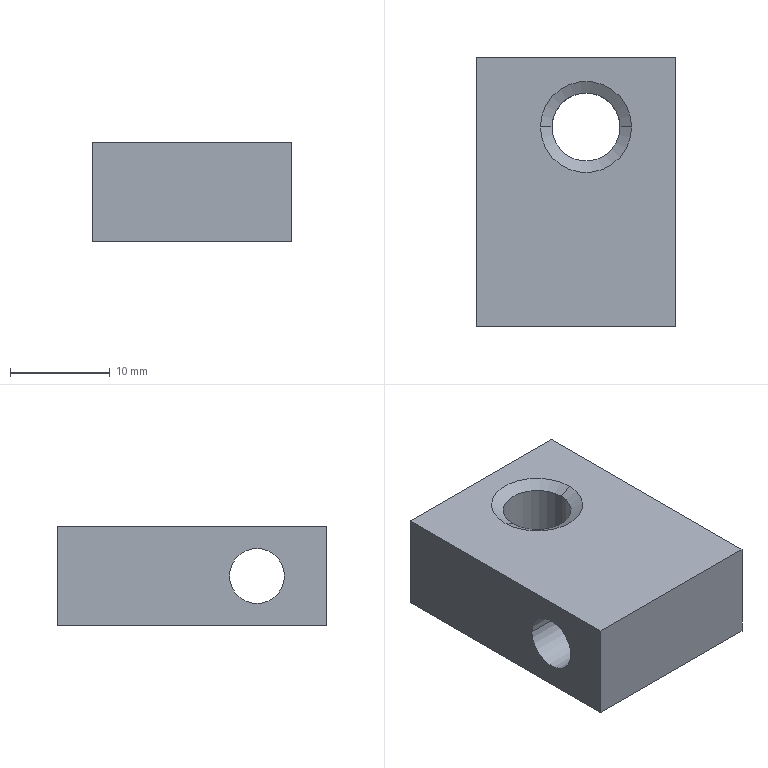Part | NX | 1 solid | 12 faces | box 20 x 27 x 10 mm | volume 4552 mm3 | plane 6 | cylinder 4 | cone 2 | commonest cylinder face diameters 5.5 x2 6.8 x2
STEP:
#1=CARTESIAN_POINT('',(508.,48.4,-222.82));
#2=VERTEX_POINT('',#1);
#3=CARTESIAN_POINT('',(508.,75.4,-222.82));
#4=VERTEX_POINT('',#3);
#5=CARTESIAN_POINT('',(508.,0.,-222.82));
#6=DIRECTION('',(0.,1.,0.));
#7=VECTOR('',#6,1000.);
#8=LINE('',#5,#7);
#9=EDGE_CURVE('',#2,#4,#8,.T.);
#10=ORIENTED_EDGE('',*,*,#9,.F.);
#11=CARTESIAN_POINT('',(528.,48.4,-222.82));
#12=VERTEX_POINT('',#11);
#13=CARTESIAN_POINT('',(0.,48.4,-222.82));
#14=DIRECTION('',(-1.,0.,0.));
#15=VECTOR('',#14,1000.);
#16=LINE('',#13,#15);
#17=EDGE_CURVE('',#12,#2,#16,.T.);
#18=ORIENTED_EDGE('',*,*,#17,.F.);
#19=CARTESIAN_POINT('',(528.,75.4,-222.82));
#20=VERTEX_POINT('',#19);
#21=CARTESIAN_POINT('',(528.,0.,-222.82));
#22=DIRECTION('',(0.,1.,0.));
#23=VECTOR('',#22,1000.);
#24=LINE('',#21,#23);
#25=EDGE_CURVE('',#12,#20,#24,.T.);
#26=ORIENTED_EDGE('',*,*,#25,.T.);
#27=CARTESIAN_POINT('',(0.,75.4,-222.82));
#28=DIRECTION('',(1.,0.,0.));
#29=VECTOR('',#28,1000.);
#30=LINE('',#27,#29);
#31=EDGE_CURVE('',#4,#20,#30,.T.);
#32=ORIENTED_EDGE('',*,*,#31,.F.);
#33=EDGE_LOOP('',(#10,#18,#26,#32));
#34=FACE_BOUND('',#33,.T.);
#35=CARTESIAN_POINT('',(523.562,68.4,-222.82));
#36=VERTEX_POINT('',#35);
#37=CARTESIAN_POINT('',(514.437,68.4,-222.82));
#38=VERTEX_POINT('',#37);
#39=CARTESIAN_POINT('',(519.,68.4,-222.82));
#40=DIRECTION('',(0.,0.,1.));
#41=DIRECTION('',(1.,0.,0.));
#42=AXIS2_PLACEMENT_3D('',#39,#40,#41);
#43=CIRCLE('',#42,4.563);
#44=EDGE_CURVE('',#36,#38,#43,.T.);
#45=ORIENTED_EDGE('',*,*,#44,.F.);
#46=CARTESIAN_POINT('',(519.,68.4,-222.82));
#47=DIRECTION('',(0.,0.,1.));
#48=DIRECTION('',(1.,0.,0.));
#49=AXIS2_PLACEMENT_3D('',#46,#47,#48);
#50=CIRCLE('',#49,4.563);
#51=EDGE_CURVE('',#38,#36,#50,.T.);
#52=ORIENTED_EDGE('',*,*,#51,.F.);
#53=EDGE_LOOP('',(#45,#52));
#54=FACE_BOUND('',#53,.T.);
#55=CARTESIAN_POINT('',(518.,48.4,-222.82));
#56=DIRECTION('',(0.,0.,1.));
#57=DIRECTION('',(1.,0.,0.));
#58=AXIS2_PLACEMENT_3D('',#55,#56,#57);
#59=PLANE('',#58);
#60=ADVANCED_FACE('',(#34,#54),#59,.T.);
#61=CARTESIAN_POINT('',(508.,48.4,-232.82));
#62=VERTEX_POINT('',#61);
#63=CARTESIAN_POINT('',(508.,48.4,-235.336));
#64=DIRECTION('',(0.,0.,1.));
#65=VECTOR('',#64,1000.);
#66=LINE('',#63,#65);
#67=EDGE_CURVE('',#62,#2,#66,.T.);
#68=ORIENTED_EDGE('',*,*,#67,.F.);
#69=CARTESIAN_POINT('',(528.,48.4,-232.82));
#70=VERTEX_POINT('',#69);
#71=CARTESIAN_POINT('',(0.,48.4,-232.82));
#72=DIRECTION('',(1.,0.,0.));
#73=VECTOR('',#72,1000.);
#74=LINE('',#71,#73);
#75=EDGE_CURVE('',#62,#70,#74,.T.);
#76=ORIENTED_EDGE('',*,*,#75,.T.);
#77=CARTESIAN_POINT('',(528.,48.4,-235.336));
#78=DIRECTION('',(0.,0.,1.));
#79=VECTOR('',#78,1000.);
#80=LINE('',#77,#79);
#81=EDGE_CURVE('',#70,#12,#80,.T.);
#82=ORIENTED_EDGE('',*,*,#81,.T.);
#83=ORIENTED_EDGE('',*,*,#17,.T.);
#84=EDGE_LOOP('',(#68,#76,#82,#83));
#85=FACE_BOUND('',#84,.T.);
#86=CARTESIAN_POINT('',(518.,48.4,-232.82));
#87=DIRECTION('',(0.,-1.,0.));
#88=DIRECTION('',(0.,0.,-1.));
#89=AXIS2_PLACEMENT_3D('',#86,#87,#88);
#90=PLANE('',#89);
#91=ADVANCED_FACE('',(#85),#90,.T.);
#92=CARTESIAN_POINT('',(508.,75.4,-232.82));
#93=VERTEX_POINT('',#92);
#94=CARTESIAN_POINT('',(508.,0.,-232.82));
#95=DIRECTION('',(0.,-1.,0.));
#96=VECTOR('',#95,1000.);
#97=LINE('',#94,#96);
#98=EDGE_CURVE('',#93,#62,#97,.T.);
#99=ORIENTED_EDGE('',*,*,#98,.F.);
#100=CARTESIAN_POINT('',(528.,75.4,-232.82));
#101=VERTEX_POINT('',#100);
#102=CARTESIAN_POINT('',(0.,75.4,-232.82));
#103=DIRECTION('',(-1.,0.,0.));
#104=VECTOR('',#103,1000.);
#105=LINE('',#102,#104);
#106=EDGE_CURVE('',#101,#93,#105,.T.);
#107=ORIENTED_EDGE('',*,*,#106,.F.);
#108=CARTESIAN_POINT('',(528.,0.,-232.82));
#109=DIRECTION('',(0.,-1.,0.));
#110=VECTOR('',#109,1000.);
#111=LINE('',#108,#110);
#112=EDGE_CURVE('',#101,#70,#111,.T.);
#113=ORIENTED_EDGE('',*,*,#112,.T.);
#114=ORIENTED_EDGE('',*,*,#75,.F.);
#115=EDGE_LOOP('',(#99,#107,#113,#114));
#116=FACE_BOUND('',#115,.T.);
#117=CARTESIAN_POINT('',(515.6,68.4,-232.82));
#118=VERTEX_POINT('',#117);
#119=CARTESIAN_POINT('',(522.4,68.4,-232.82));
#120=VERTEX_POINT('',#119);
#121=CARTESIAN_POINT('',(519.,68.4,-232.82));
#122=DIRECTION('',(0.,0.,1.));
#123=DIRECTION('',(1.,0.,0.));
#124=AXIS2_PLACEMENT_3D('',#121,#122,#123);
#125=CIRCLE('',#124,3.4);
#126=EDGE_CURVE('',#118,#120,#125,.T.);
#127=ORIENTED_EDGE('',*,*,#126,.T.);
#128=CARTESIAN_POINT('',(519.,68.4,-232.82));
#129=DIRECTION('',(0.,0.,1.));
#130=DIRECTION('',(1.,0.,0.));
#131=AXIS2_PLACEMENT_3D('',#128,#129,#130);
#132=CIRCLE('',#131,3.4);
#133=EDGE_CURVE('',#120,#118,#132,.T.);
#134=ORIENTED_EDGE('',*,*,#133,.T.);
#135=EDGE_LOOP('',(#127,#134));
#136=FACE_BOUND('',#135,.T.);
#137=CARTESIAN_POINT('',(518.,62.4,-232.82));
#138=DIRECTION('',(0.,0.,-1.));
#139=DIRECTION('',(0.,-1.,0.));
#140=AXIS2_PLACEMENT_3D('',#137,#138,#139);
#141=PLANE('',#140);
#142=ADVANCED_FACE('',(#116,#136),#141,.T.);
#143=CARTESIAN_POINT('',(508.,75.4,-235.336));
#144=DIRECTION('',(0.,0.,-1.));
#145=VECTOR('',#144,1000.);
#146=LINE('',#143,#145);
#147=EDGE_CURVE('',#4,#93,#146,.T.);
#148=ORIENTED_EDGE('',*,*,#147,.F.);
#149=ORIENTED_EDGE('',*,*,#31,.T.);
#150=CARTESIAN_POINT('',(528.,75.4,-235.336));
#151=DIRECTION('',(0.,0.,1.));
#152=VECTOR('',#151,1000.);
#153=LINE('',#150,#152);
#154=EDGE_CURVE('',#101,#20,#153,.T.);
#155=ORIENTED_EDGE('',*,*,#154,.F.);
#156=ORIENTED_EDGE('',*,*,#106,.T.);
#157=EDGE_LOOP('',(#148,#149,#155,#156));
#158=FACE_BOUND('',#157,.T.);
#159=CARTESIAN_POINT('',(518.,75.4,-222.82));
#160=DIRECTION('',(0.,1.,0.));
#161=DIRECTION('',(1.,0.,0.));
#162=AXIS2_PLACEMENT_3D('',#159,#160,#161);
#163=PLANE('',#162);
#164=ADVANCED_FACE('',(#158),#163,.T.);
#165=ORIENTED_EDGE('',*,*,#98,.T.);
#166=ORIENTED_EDGE('',*,*,#67,.T.);
#167=ORIENTED_EDGE('',*,*,#9,.T.);
#168=ORIENTED_EDGE('',*,*,#147,.T.);
#169=EDGE_LOOP('',(#165,#166,#167,#168));
#170=FACE_BOUND('',#169,.T.);
#171=CARTESIAN_POINT('',(508.,52.65,-227.82));
#172=VERTEX_POINT('',#171);
#173=CARTESIAN_POINT('',(508.,58.15,-227.82));
#174=VERTEX_POINT('',#173);
#175=CARTESIAN_POINT('',(508.,55.4,-227.82));
#176=DIRECTION('',(-1.,0.,0.));
#177=DIRECTION('',(0.,-1.,0.));
#178=AXIS2_PLACEMENT_3D('',#175,#176,#177);
#179=CIRCLE('',#178,2.75);
#180=EDGE_CURVE('',#172,#174,#179,.T.);
#181=ORIENTED_EDGE('',*,*,#180,.F.);
#182=CARTESIAN_POINT('',(508.,55.4,-227.82));
#183=DIRECTION('',(-1.,0.,0.));
#184=DIRECTION('',(0.,-1.,0.));
#185=AXIS2_PLACEMENT_3D('',#182,#183,#184);
#186=CIRCLE('',#185,2.75);
#187=EDGE_CURVE('',#174,#172,#186,.T.);
#188=ORIENTED_EDGE('',*,*,#187,.F.);
#189=EDGE_LOOP('',(#181,#188));
#190=FACE_BOUND('',#189,.T.);
#191=CARTESIAN_POINT('',(508.,57.102,-235.336));
#192=DIRECTION('',(-1.,0.,0.));
#193=DIRECTION('',(0.,1.,0.));
#194=AXIS2_PLACEMENT_3D('',#191,#192,#193);
#195=PLANE('',#194);
#196=ADVANCED_FACE('',(#170,#190),#195,.T.);
#197=ORIENTED_EDGE('',*,*,#154,.T.);
#198=ORIENTED_EDGE('',*,*,#25,.F.);
#199=ORIENTED_EDGE('',*,*,#81,.F.);
#200=ORIENTED_EDGE('',*,*,#112,.F.);
#201=EDGE_LOOP('',(#197,#198,#199,#200));
#202=FACE_BOUND('',#201,.T.);
#203=CARTESIAN_POINT('',(528.,52.65,-227.82));
#204=VERTEX_POINT('',#203);
#205=CARTESIAN_POINT('',(528.,58.15,-227.82));
#206=VERTEX_POINT('',#205);
#207=CARTESIAN_POINT('',(528.,55.4,-227.82));
#208=DIRECTION('',(-1.,0.,0.));
#209=DIRECTION('',(0.,-1.,0.));
#210=AXIS2_PLACEMENT_3D('',#207,#208,#209);
#211=CIRCLE('',#210,2.75);
#212=EDGE_CURVE('',#204,#206,#211,.T.);
#213=ORIENTED_EDGE('',*,*,#212,.T.);
#214=CARTESIAN_POINT('',(528.,55.4,-227.82));
#215=DIRECTION('',(-1.,0.,0.));
#216=DIRECTION('',(0.,-1.,0.));
#217=AXIS2_PLACEMENT_3D('',#214,#215,#216);
#218=CIRCLE('',#217,2.75);
#219=EDGE_CURVE('',#206,#204,#218,.T.);
#220=ORIENTED_EDGE('',*,*,#219,.T.);
#221=EDGE_LOOP('',(#213,#220));
#222=FACE_BOUND('',#221,.T.);
#223=CARTESIAN_POINT('',(528.,57.102,-235.336));
#224=DIRECTION('',(-1.,0.,0.));
#225=DIRECTION('',(0.,1.,0.));
#226=AXIS2_PLACEMENT_3D('',#223,#224,#225);
#227=PLANE('',#226);
#228=ADVANCED_FACE('',(#202,#222),#227,.F.);
#229=ORIENTED_EDGE('',*,*,#212,.F.);
#230=CARTESIAN_POINT('',(521.2,52.65,-227.82));
#231=DIRECTION('',(-1.,0.,0.));
#232=VECTOR('',#231,1000.);
#233=LINE('',#230,#232);
#234=EDGE_CURVE('',#172,#204,#233,.F.);
#235=ORIENTED_EDGE('',*,*,#234,.F.);
#236=ORIENTED_EDGE('',*,*,#180,.T.);
#237=CARTESIAN_POINT('',(521.2,58.15,-227.82));
#238=DIRECTION('',(-1.,0.,0.));
#239=VECTOR('',#238,1000.);
#240=LINE('',#237,#239);
#241=EDGE_CURVE('',#174,#206,#240,.F.);
#242=ORIENTED_EDGE('',*,*,#241,.T.);
#243=EDGE_LOOP('',(#229,#235,#236,#242));
#244=FACE_BOUND('',#243,.T.);
#245=CARTESIAN_POINT('',(521.2,55.4,-227.82));
#246=DIRECTION('',(-1.,0.,0.));
#247=DIRECTION('',(0.,-1.,0.));
#248=AXIS2_PLACEMENT_3D('',#245,#246,#247);
#249=CYLINDRICAL_SURFACE('',#248,2.75);
#250=ADVANCED_FACE('',(#244),#249,.F.);
#251=ORIENTED_EDGE('',*,*,#126,.F.);
#252=CARTESIAN_POINT('',(515.6,68.4,-223.491));
#253=VERTEX_POINT('',#252);
#254=CARTESIAN_POINT('',(515.6,68.4,-222.82));
#255=DIRECTION('',(0.,0.,1.));
#256=VECTOR('',#255,1000.);
#257=LINE('',#254,#256);
#258=EDGE_CURVE('',#118,#253,#257,.T.);
#259=ORIENTED_EDGE('',*,*,#258,.T.);
#260=CARTESIAN_POINT('',(522.4,68.4,-223.491));
#261=VERTEX_POINT('',#260);
#262=CARTESIAN_POINT('',(519.,68.4,-223.491));
#263=DIRECTION('',(0.,0.,1.));
#264=DIRECTION('',(1.,0.,0.));
#265=AXIS2_PLACEMENT_3D('',#262,#263,#264);
#266=CIRCLE('',#265,3.4);
#267=EDGE_CURVE('',#253,#261,#266,.T.);
#268=ORIENTED_EDGE('',*,*,#267,.T.);
#269=CARTESIAN_POINT('',(522.4,68.4,-222.82));
#270=DIRECTION('',(0.,0.,1.));
#271=VECTOR('',#270,1000.);
#272=LINE('',#269,#271);
#273=EDGE_CURVE('',#120,#261,#272,.T.);
#274=ORIENTED_EDGE('',*,*,#273,.F.);
#275=EDGE_LOOP('',(#251,#259,#268,#274));
#276=FACE_BOUND('',#275,.T.);
#277=CARTESIAN_POINT('',(519.,68.4,-222.82));
#278=DIRECTION('',(0.,0.,1.));
#279=DIRECTION('',(1.,0.,0.));
#280=AXIS2_PLACEMENT_3D('',#277,#278,#279);
#281=CYLINDRICAL_SURFACE('',#280,3.4);
#282=ADVANCED_FACE('',(#276),#281,.F.);
#283=ORIENTED_EDGE('',*,*,#267,.F.);
#284=CARTESIAN_POINT('',(515.6,68.4,-223.491));
#285=DIRECTION('',(-0.866,0.,0.5));
#286=VECTOR('',#285,1000.);
#287=LINE('',#284,#286);
#288=EDGE_CURVE('',#38,#253,#287,.F.);
#289=ORIENTED_EDGE('',*,*,#288,.F.);
#290=ORIENTED_EDGE('',*,*,#51,.T.);
#291=CARTESIAN_POINT('',(522.4,68.4,-223.491));
#292=DIRECTION('',(0.866,0.,0.5));
#293=VECTOR('',#292,1000.);
#294=LINE('',#291,#293);
#295=EDGE_CURVE('',#36,#261,#294,.F.);
#296=ORIENTED_EDGE('',*,*,#295,.T.);
#297=EDGE_LOOP('',(#283,#289,#290,#296));
#298=FACE_BOUND('',#297,.T.);
#299=CARTESIAN_POINT('',(519.,68.4,-223.491));
#300=DIRECTION('',(0.,0.,1.));
#301=DIRECTION('',(1.,0.,0.));
#302=AXIS2_PLACEMENT_3D('',#299,#300,#301);
#303=CONICAL_SURFACE('',#302,3.4,1.047);
#304=ADVANCED_FACE('',(#298),#303,.F.);
#305=ORIENTED_EDGE('',*,*,#273,.T.);
#306=CARTESIAN_POINT('',(519.,68.4,-223.491));
#307=DIRECTION('',(0.,0.,1.));
#308=DIRECTION('',(1.,0.,0.));
#309=AXIS2_PLACEMENT_3D('',#306,#307,#308);
#310=CIRCLE('',#309,3.4);
#311=EDGE_CURVE('',#261,#253,#310,.T.);
#312=ORIENTED_EDGE('',*,*,#311,.T.);
#313=ORIENTED_EDGE('',*,*,#258,.F.);
#314=ORIENTED_EDGE('',*,*,#133,.F.);
#315=EDGE_LOOP('',(#305,#312,#313,#314));
#316=FACE_BOUND('',#315,.T.);
#317=CARTESIAN_POINT('',(519.,68.4,-222.82));
#318=DIRECTION('',(0.,0.,1.));
#319=DIRECTION('',(1.,0.,0.));
#320=AXIS2_PLACEMENT_3D('',#317,#318,#319);
#321=CYLINDRICAL_SURFACE('',#320,3.4);
#322=ADVANCED_FACE('',(#316),#321,.F.);
#323=ORIENTED_EDGE('',*,*,#234,.T.);
#324=ORIENTED_EDGE('',*,*,#219,.F.);
#325=ORIENTED_EDGE('',*,*,#241,.F.);
#326=ORIENTED_EDGE('',*,*,#187,.T.);
#327=EDGE_LOOP('',(#323,#324,#325,#326));
#328=FACE_BOUND('',#327,.T.);
#329=CARTESIAN_POINT('',(521.2,55.4,-227.82));
#330=DIRECTION('',(-1.,0.,0.));
#331=DIRECTION('',(0.,-1.,0.));
#332=AXIS2_PLACEMENT_3D('',#329,#330,#331);
#333=CYLINDRICAL_SURFACE('',#332,2.75);
#334=ADVANCED_FACE('',(#328),#333,.F.);
#335=ORIENTED_EDGE('',*,*,#44,.T.);
#336=ORIENTED_EDGE('',*,*,#288,.T.);
#337=ORIENTED_EDGE('',*,*,#311,.F.);
#338=ORIENTED_EDGE('',*,*,#295,.F.);
#339=EDGE_LOOP('',(#335,#336,#337,#338));
#340=FACE_BOUND('',#339,.T.);
#341=CARTESIAN_POINT('',(519.,68.4,-223.491));
#342=DIRECTION('',(0.,0.,1.));
#343=DIRECTION('',(1.,0.,0.));
#344=AXIS2_PLACEMENT_3D('',#341,#342,#343);
#345=CONICAL_SURFACE('',#344,3.4,1.047);
#346=ADVANCED_FACE('',(#340),#345,.F.);
#347=CLOSED_SHELL('',(#60,#91,#142,#164,#196,#228,#250,#282,#304,#322,#334,#346));
#348=MANIFOLD_SOLID_BREP('',#347);
#349=(LENGTH_UNIT()NAMED_UNIT(*)SI_UNIT(.MILLI.,.METRE.));
#350=UNCERTAINTY_MEASURE_WITH_UNIT(LENGTH_MEASURE(0.00001),#349,'','');
#351=(NAMED_UNIT(*)PLANE_ANGLE_UNIT()SI_UNIT($,.RADIAN.));
#352=(NAMED_UNIT(*)SI_UNIT($,.STERADIAN.)SOLID_ANGLE_UNIT());
#353=(GEOMETRIC_REPRESENTATION_CONTEXT(3)GLOBAL_UNCERTAINTY_ASSIGNED_CONTEXT((#350))GLOBAL_UNIT_ASSIGNED_CONTEXT((#349,#351,#352))REPRESENTATION_CONTEXT('',''));
#354=ADVANCED_BREP_SHAPE_REPRESENTATION('',(#348),#353);